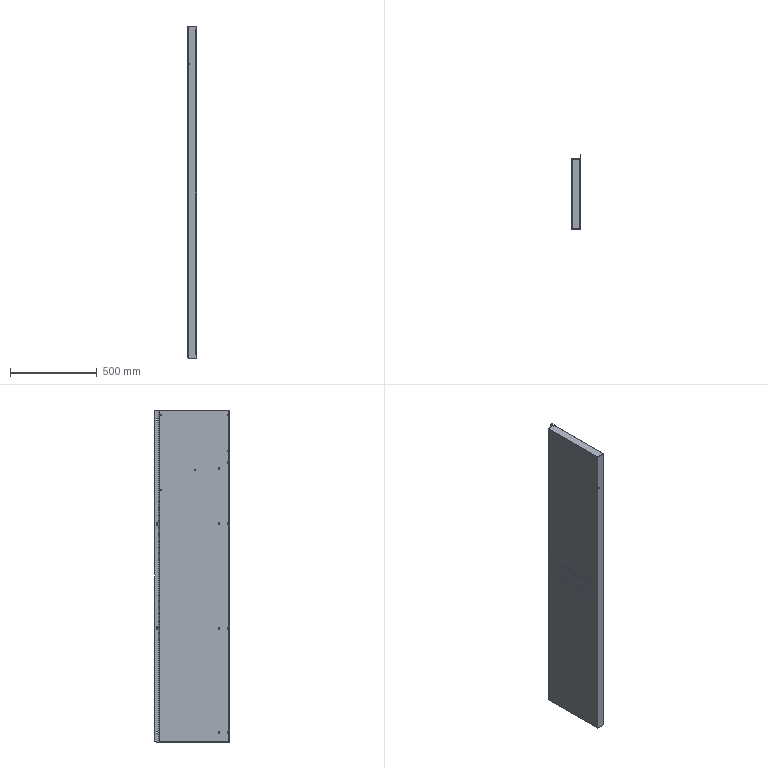Part | SolidWorks | 2 solids | 210 faces | box 50 x 430 x 1914 mm | volume 1776618 mm3 | plane 130 | cylinder 76 | spline 4 | commonest cylinder face diameters 6 x14 2 x13 5 x13 6.4 x12 7 x12 8 x8